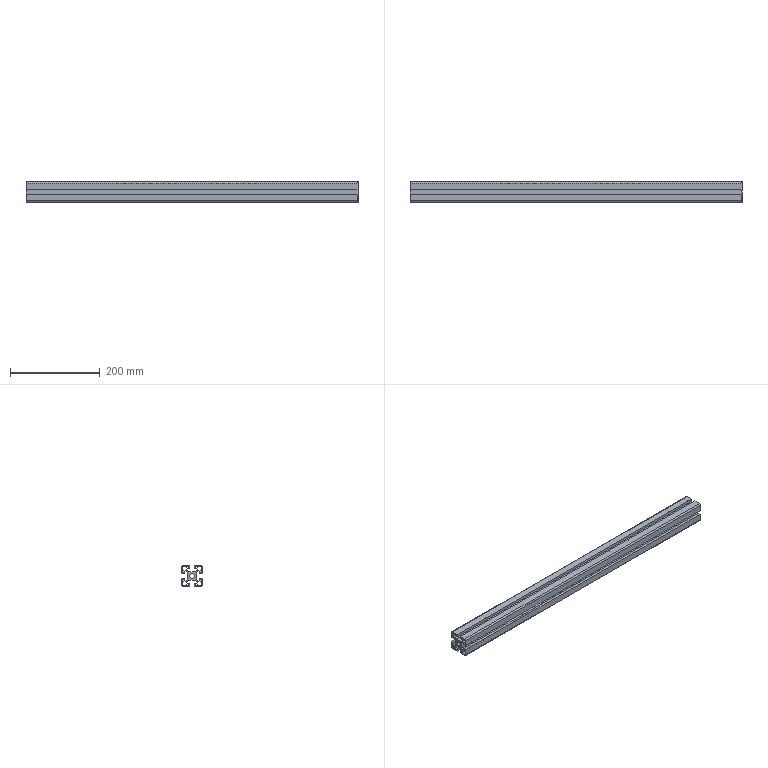Part | STEP file | bosch_3842990520_1jcimurca0n3y5im9bxpmvpzt | 1 solid | 87 faces | box 740 x 45 x 45 mm | volume 605130 mm3 | plane 78 | cylinder 9 | commonest cylinder face diameters 2 x4 6 x4 10 x1